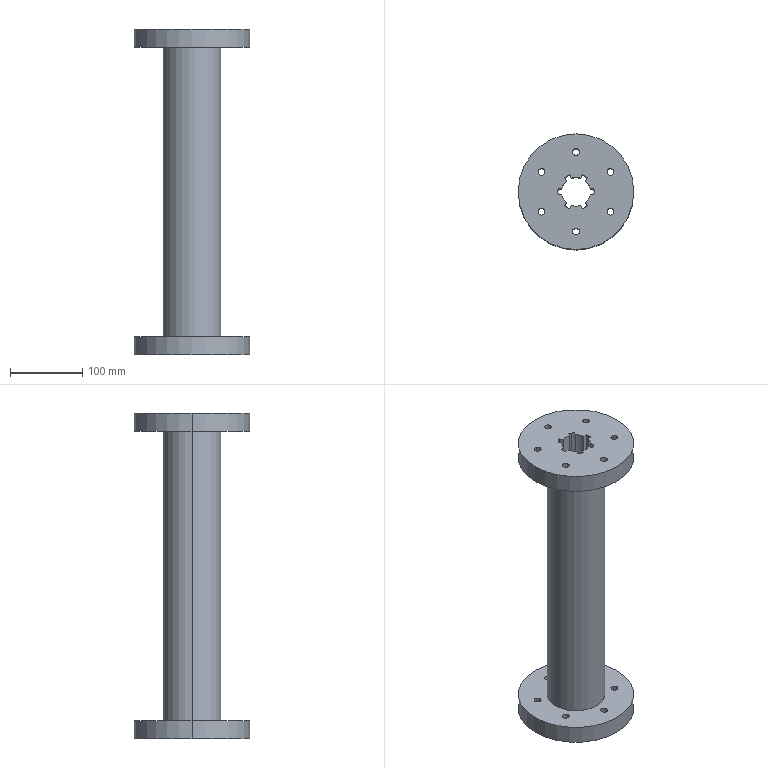Part | SolidWorks | features BaseBody 1 | 1 solid | 64 faces | box 160 x 160 x 450 mm | volume 2320559 mm3 | cylinder 48 | plane 16 | commonest cylinder face diameters 9.508 x24 50 x12 40 x6 160 x4 80 x2